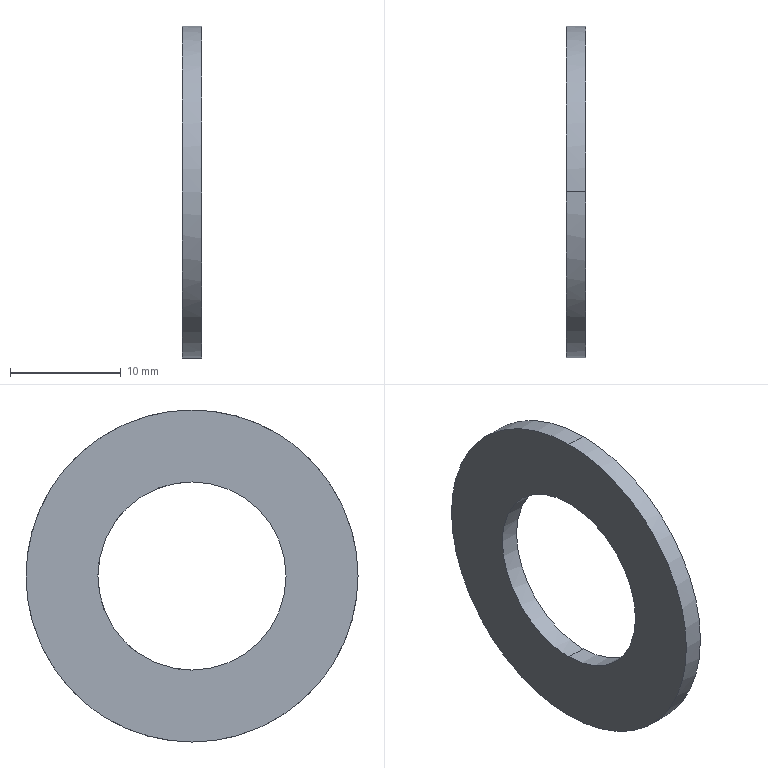Part | STEP file | _SPWF16 | 1 solid | 6 faces | box 1.8 x 30 x 30 mm | volume 863.783 mm3 | cylinder 4 | plane 2 | commonest cylinder face diameters 17 x2 30 x2
STEP:
#1=CARTESIAN_POINT('',(-0.3,0.,-8.5));
#2=VERTEX_POINT('',#1);
#3=CARTESIAN_POINT('',(1.5,0.,-8.5));
#4=VERTEX_POINT('',#3);
#5=CARTESIAN_POINT('',(1.5,0.,-8.5));
#6=DIRECTION('',(-1.,0.,0.));
#7=VECTOR('',#6,1.);
#8=LINE('',#5,#7);
#9=EDGE_CURVE('',#2,#4,#8,.F.);
#10=ORIENTED_EDGE('',*,*,#9,.F.);
#11=CARTESIAN_POINT('',(-0.3,-8.5,0.));
#12=VERTEX_POINT('',#11);
#13=CARTESIAN_POINT('',(-0.3,0.,0.));
#14=DIRECTION('',(-1.,0.,0.));
#15=AXIS2_PLACEMENT_3D('',#13,#14,$);
#16=CIRCLE('',#15,8.5);
#17=EDGE_CURVE('',#12,#2,#16,.F.);
#18=ORIENTED_EDGE('',*,*,#17,.F.);
#19=CARTESIAN_POINT('',(-0.3,0.,8.5));
#20=VERTEX_POINT('',#19);
#21=CARTESIAN_POINT('',(-0.3,0.,0.));
#22=DIRECTION('',(-1.,0.,0.));
#23=AXIS2_PLACEMENT_3D('',#21,#22,$);
#24=CIRCLE('',#23,8.5);
#25=EDGE_CURVE('',#20,#12,#24,.F.);
#26=ORIENTED_EDGE('',*,*,#25,.F.);
#27=CARTESIAN_POINT('',(1.5,0.,8.5));
#28=VERTEX_POINT('',#27);
#29=CARTESIAN_POINT('',(1.5,0.,8.5));
#30=DIRECTION('',(-1.,0.,0.));
#31=VECTOR('',#30,1.);
#32=LINE('',#29,#31);
#33=EDGE_CURVE('',#28,#20,#32,.T.);
#34=ORIENTED_EDGE('',*,*,#33,.F.);
#35=CARTESIAN_POINT('',(1.5,-8.5,0.));
#36=VERTEX_POINT('',#35);
#37=CARTESIAN_POINT('',(1.5,0.,0.));
#38=DIRECTION('',(-1.,0.,0.));
#39=AXIS2_PLACEMENT_3D('',#37,#38,$);
#40=CIRCLE('',#39,8.5);
#41=EDGE_CURVE('',#28,#36,#40,.F.);
#42=ORIENTED_EDGE('',*,*,#41,.T.);
#43=CARTESIAN_POINT('',(1.5,0.,0.));
#44=DIRECTION('',(-1.,0.,0.));
#45=AXIS2_PLACEMENT_3D('',#43,#44,$);
#46=CIRCLE('',#45,8.5);
#47=EDGE_CURVE('',#36,#4,#46,.F.);
#48=ORIENTED_EDGE('',*,*,#47,.T.);
#49=EDGE_LOOP('',(#10,#18,#26,#34,#42,#48));
#50=FACE_OUTER_BOUND('',#49,.T.);
#51=CARTESIAN_POINT('',(1.5,0.,0.));
#52=DIRECTION('',(-1.,0.,0.));
#53=DIRECTION('',(0.,0.,-1.));
#54=AXIS2_PLACEMENT_3D('',#51,#52,#53);
#55=CYLINDRICAL_SURFACE('',#54,8.5);
#56=ADVANCED_FACE('',(#50),#55,.F.);
#57=CARTESIAN_POINT('',(-0.3,0.,15.));
#58=VERTEX_POINT('',#57);
#59=CARTESIAN_POINT('',(-0.3,-15.,0.));
#60=VERTEX_POINT('',#59);
#61=CARTESIAN_POINT('',(-0.3,-15.,0.));
#62=CARTESIAN_POINT('',(-0.3,-15.,4.712));
#63=CARTESIAN_POINT('',(-0.3,-13.155,9.429));
#64=CARTESIAN_POINT('',(-0.3,-9.429,13.155));
#65=CARTESIAN_POINT('',(-0.3,-4.712,15.));
#66=CARTESIAN_POINT('',(-0.3,0.,15.));
#67=B_SPLINE_CURVE_WITH_KNOTS('',5,(#61,#62,#63,#64,#65,#66),.UNSPECIFIED.,.F.,.U.,(6,6),(70.686,94.248),.UNSPECIFIED.);
#68=EDGE_CURVE('',#58,#60,#67,.F.);
#69=ORIENTED_EDGE('',*,*,#68,.F.);
#70=CARTESIAN_POINT('',(-0.3,15.,0.));
#71=VERTEX_POINT('',#70);
#72=CARTESIAN_POINT('',(-0.3,0.,15.));
#73=CARTESIAN_POINT('',(-0.3,4.712,15.));
#74=CARTESIAN_POINT('',(-0.3,9.429,13.155));
#75=CARTESIAN_POINT('',(-0.3,13.155,9.429));
#76=CARTESIAN_POINT('',(-0.3,15.,4.712));
#77=CARTESIAN_POINT('',(-0.3,15.,0.));
#78=B_SPLINE_CURVE_WITH_KNOTS('',5,(#72,#73,#74,#75,#76,#77),.UNSPECIFIED.,.F.,.U.,(6,6),(0.,23.562),.UNSPECIFIED.);
#79=EDGE_CURVE('',#71,#58,#78,.F.);
#80=ORIENTED_EDGE('',*,*,#79,.F.);
#81=CARTESIAN_POINT('',(-0.3,0.,-15.));
#82=VERTEX_POINT('',#81);
#83=CARTESIAN_POINT('',(-0.3,15.,0.));
#84=CARTESIAN_POINT('',(-0.3,15.,-4.712));
#85=CARTESIAN_POINT('',(-0.3,13.155,-9.429));
#86=CARTESIAN_POINT('',(-0.3,9.429,-13.155));
#87=CARTESIAN_POINT('',(-0.3,4.712,-15.));
#88=CARTESIAN_POINT('',(-0.3,0.,-15.));
#89=B_SPLINE_CURVE_WITH_KNOTS('',5,(#83,#84,#85,#86,#87,#88),.UNSPECIFIED.,.F.,.U.,(6,6),(23.562,47.124),.UNSPECIFIED.);
#90=EDGE_CURVE('',#82,#71,#89,.F.);
#91=ORIENTED_EDGE('',*,*,#90,.F.);
#92=CARTESIAN_POINT('',(-0.3,0.,-15.));
#93=CARTESIAN_POINT('',(-0.3,-4.712,-15.));
#94=CARTESIAN_POINT('',(-0.3,-9.429,-13.155));
#95=CARTESIAN_POINT('',(-0.3,-13.155,-9.429));
#96=CARTESIAN_POINT('',(-0.3,-15.,-4.712));
#97=CARTESIAN_POINT('',(-0.3,-15.,0.));
#98=B_SPLINE_CURVE_WITH_KNOTS('',5,(#92,#93,#94,#95,#96,#97),.UNSPECIFIED.,.F.,.U.,(6,6),(47.124,70.686),.UNSPECIFIED.);
#99=EDGE_CURVE('',#60,#82,#98,.F.);
#100=ORIENTED_EDGE('',*,*,#99,.F.);
#101=EDGE_LOOP('',(#69,#80,#91,#100));
#102=FACE_OUTER_BOUND('',#101,.T.);
#103=CARTESIAN_POINT('',(-0.3,8.5,0.));
#104=VERTEX_POINT('',#103);
#105=CARTESIAN_POINT('',(-0.3,8.5,0.));
#106=CARTESIAN_POINT('',(-0.3,8.5,-2.67));
#107=CARTESIAN_POINT('',(-0.3,7.454,-5.343));
#108=CARTESIAN_POINT('',(-0.3,5.343,-7.454));
#109=CARTESIAN_POINT('',(-0.3,2.67,-8.5));
#110=CARTESIAN_POINT('',(-0.3,0.,-8.5));
#111=B_SPLINE_CURVE_WITH_KNOTS('',5,(#105,#106,#107,#108,#109,#110),.UNSPECIFIED.,.F.,.U.,(6,6),(13.352,26.704),.UNSPECIFIED.);
#112=EDGE_CURVE('',#2,#104,#111,.F.);
#113=ORIENTED_EDGE('',*,*,#112,.T.);
#114=CARTESIAN_POINT('',(-0.3,0.,8.5));
#115=CARTESIAN_POINT('',(-0.3,2.67,8.5));
#116=CARTESIAN_POINT('',(-0.3,5.343,7.454));
#117=CARTESIAN_POINT('',(-0.3,7.454,5.343));
#118=CARTESIAN_POINT('',(-0.3,8.5,2.67));
#119=CARTESIAN_POINT('',(-0.3,8.5,0.));
#120=B_SPLINE_CURVE_WITH_KNOTS('',5,(#114,#115,#116,#117,#118,#119),.UNSPECIFIED.,.F.,.U.,(6,6),(0.,13.352),.UNSPECIFIED.);
#121=EDGE_CURVE('',#104,#20,#120,.F.);
#122=ORIENTED_EDGE('',*,*,#121,.T.);
#123=ORIENTED_EDGE('',*,*,#25,.T.);
#124=ORIENTED_EDGE('',*,*,#17,.T.);
#125=EDGE_LOOP('',(#113,#122,#123,#124));
#126=FACE_BOUND('',#125,.T.);
#127=CARTESIAN_POINT('',(-0.3,15.,0.));
#128=DIRECTION('',(-1.,0.,0.));
#129=DIRECTION('',(0.,0.,1.));
#130=AXIS2_PLACEMENT_3D('',#127,#128,#129);
#131=PLANE('',#130);
#132=ADVANCED_FACE('',(#102,#126),#131,.T.);
#133=ORIENTED_EDGE('',*,*,#99,.T.);
#134=CARTESIAN_POINT('',(1.5,0.,-15.));
#135=VERTEX_POINT('',#134);
#136=CARTESIAN_POINT('',(1.5,0.,-15.));
#137=DIRECTION('',(-1.,0.,0.));
#138=VECTOR('',#137,1.);
#139=LINE('',#136,#138);
#140=EDGE_CURVE('',#82,#135,#139,.F.);
#141=ORIENTED_EDGE('',*,*,#140,.T.);
#142=CARTESIAN_POINT('',(1.5,-15.,0.));
#143=VERTEX_POINT('',#142);
#144=CARTESIAN_POINT('',(1.5,0.,0.));
#145=DIRECTION('',(-1.,0.,0.));
#146=AXIS2_PLACEMENT_3D('',#144,#145,$);
#147=CIRCLE('',#146,15.);
#148=EDGE_CURVE('',#143,#135,#147,.F.);
#149=ORIENTED_EDGE('',*,*,#148,.F.);
#150=CARTESIAN_POINT('',(1.5,0.,15.));
#151=VERTEX_POINT('',#150);
#152=CARTESIAN_POINT('',(1.5,0.,0.));
#153=DIRECTION('',(-1.,0.,0.));
#154=AXIS2_PLACEMENT_3D('',#152,#153,$);
#155=CIRCLE('',#154,15.);
#156=EDGE_CURVE('',#151,#143,#155,.F.);
#157=ORIENTED_EDGE('',*,*,#156,.F.);
#158=CARTESIAN_POINT('',(1.5,0.,15.));
#159=DIRECTION('',(-1.,0.,0.));
#160=VECTOR('',#159,1.);
#161=LINE('',#158,#160);
#162=EDGE_CURVE('',#151,#58,#161,.T.);
#163=ORIENTED_EDGE('',*,*,#162,.T.);
#164=ORIENTED_EDGE('',*,*,#68,.T.);
#165=EDGE_LOOP('',(#133,#141,#149,#157,#163,#164));
#166=FACE_OUTER_BOUND('',#165,.T.);
#167=CARTESIAN_POINT('',(1.5,0.,0.));
#168=DIRECTION('',(-1.,0.,0.));
#169=DIRECTION('',(0.,0.,-1.));
#170=AXIS2_PLACEMENT_3D('',#167,#168,#169);
#171=CYLINDRICAL_SURFACE('',#170,15.);
#172=ADVANCED_FACE('',(#166),#171,.T.);
#173=ORIENTED_EDGE('',*,*,#79,.T.);
#174=ORIENTED_EDGE('',*,*,#162,.F.);
#175=CARTESIAN_POINT('',(1.5,15.,0.));
#176=VERTEX_POINT('',#175);
#177=CARTESIAN_POINT('',(1.5,0.,0.));
#178=DIRECTION('',(-1.,0.,0.));
#179=AXIS2_PLACEMENT_3D('',#177,#178,$);
#180=CIRCLE('',#179,15.);
#181=EDGE_CURVE('',#176,#151,#180,.F.);
#182=ORIENTED_EDGE('',*,*,#181,.F.);
#183=CARTESIAN_POINT('',(1.5,0.,0.));
#184=DIRECTION('',(-1.,0.,0.));
#185=AXIS2_PLACEMENT_3D('',#183,#184,$);
#186=CIRCLE('',#185,15.);
#187=EDGE_CURVE('',#135,#176,#186,.F.);
#188=ORIENTED_EDGE('',*,*,#187,.F.);
#189=ORIENTED_EDGE('',*,*,#140,.F.);
#190=ORIENTED_EDGE('',*,*,#90,.T.);
#191=EDGE_LOOP('',(#173,#174,#182,#188,#189,#190));
#192=FACE_OUTER_BOUND('',#191,.T.);
#193=CARTESIAN_POINT('',(1.5,0.,0.));
#194=DIRECTION('',(-1.,0.,0.));
#195=DIRECTION('',(0.,0.,1.));
#196=AXIS2_PLACEMENT_3D('',#193,#194,#195);
#197=CYLINDRICAL_SURFACE('',#196,15.);
#198=ADVANCED_FACE('',(#192),#197,.T.);
#199=ORIENTED_EDGE('',*,*,#181,.T.);
#200=ORIENTED_EDGE('',*,*,#156,.T.);
#201=ORIENTED_EDGE('',*,*,#148,.T.);
#202=ORIENTED_EDGE('',*,*,#187,.T.);
#203=EDGE_LOOP('',(#199,#200,#201,#202));
#204=FACE_OUTER_BOUND('',#203,.T.);
#205=CARTESIAN_POINT('',(1.5,8.5,0.));
#206=VERTEX_POINT('',#205);
#207=CARTESIAN_POINT('',(1.5,0.,0.));
#208=DIRECTION('',(1.,0.,0.));
#209=AXIS2_PLACEMENT_3D('',#207,#208,$);
#210=CIRCLE('',#209,8.5);
#211=EDGE_CURVE('',#4,#206,#210,.T.);
#212=ORIENTED_EDGE('',*,*,#211,.F.);
#213=ORIENTED_EDGE('',*,*,#47,.F.);
#214=ORIENTED_EDGE('',*,*,#41,.F.);
#215=CARTESIAN_POINT('',(1.5,0.,0.));
#216=DIRECTION('',(1.,0.,0.));
#217=AXIS2_PLACEMENT_3D('',#215,#216,$);
#218=CIRCLE('',#217,8.5);
#219=EDGE_CURVE('',#206,#28,#218,.T.);
#220=ORIENTED_EDGE('',*,*,#219,.F.);
#221=EDGE_LOOP('',(#212,#213,#214,#220));
#222=FACE_BOUND('',#221,.T.);
#223=CARTESIAN_POINT('',(1.5,8.5,0.));
#224=DIRECTION('',(1.,0.,0.));
#225=DIRECTION('',(0.,0.,-1.));
#226=AXIS2_PLACEMENT_3D('',#223,#224,#225);
#227=PLANE('',#226);
#228=ADVANCED_FACE('',(#204,#222),#227,.T.);
#229=ORIENTED_EDGE('',*,*,#211,.T.);
#230=ORIENTED_EDGE('',*,*,#219,.T.);
#231=ORIENTED_EDGE('',*,*,#33,.T.);
#232=ORIENTED_EDGE('',*,*,#121,.F.);
#233=ORIENTED_EDGE('',*,*,#112,.F.);
#234=ORIENTED_EDGE('',*,*,#9,.T.);
#235=EDGE_LOOP('',(#229,#230,#231,#232,#233,#234));
#236=FACE_OUTER_BOUND('',#235,.T.);
#237=CARTESIAN_POINT('',(1.5,0.,0.));
#238=DIRECTION('',(-1.,0.,0.));
#239=DIRECTION('',(0.,0.,1.));
#240=AXIS2_PLACEMENT_3D('',#237,#238,#239);
#241=CYLINDRICAL_SURFACE('',#240,8.5);
#242=ADVANCED_FACE('',(#236),#241,.F.);
#243=CLOSED_SHELL('',(#56,#132,#172,#198,#228,#242));
#244=MANIFOLD_SOLID_BREP('',#243);
#245=(LENGTH_UNIT()NAMED_UNIT(*)SI_UNIT(.MILLI.,.METRE.));
#246=UNCERTAINTY_MEASURE_WITH_UNIT(LENGTH_MEASURE(0.005),#245,'','');
#247=(NAMED_UNIT(*)PLANE_ANGLE_UNIT()SI_UNIT($,.RADIAN.));
#248=(NAMED_UNIT(*)SI_UNIT($,.STERADIAN.)SOLID_ANGLE_UNIT());
#249=(GEOMETRIC_REPRESENTATION_CONTEXT(3)GLOBAL_UNCERTAINTY_ASSIGNED_CONTEXT((#246))GLOBAL_UNIT_ASSIGNED_CONTEXT((#245,#247,#248))REPRESENTATION_CONTEXT('',''));
#250=ADVANCED_BREP_SHAPE_REPRESENTATION('',(#244),#249);